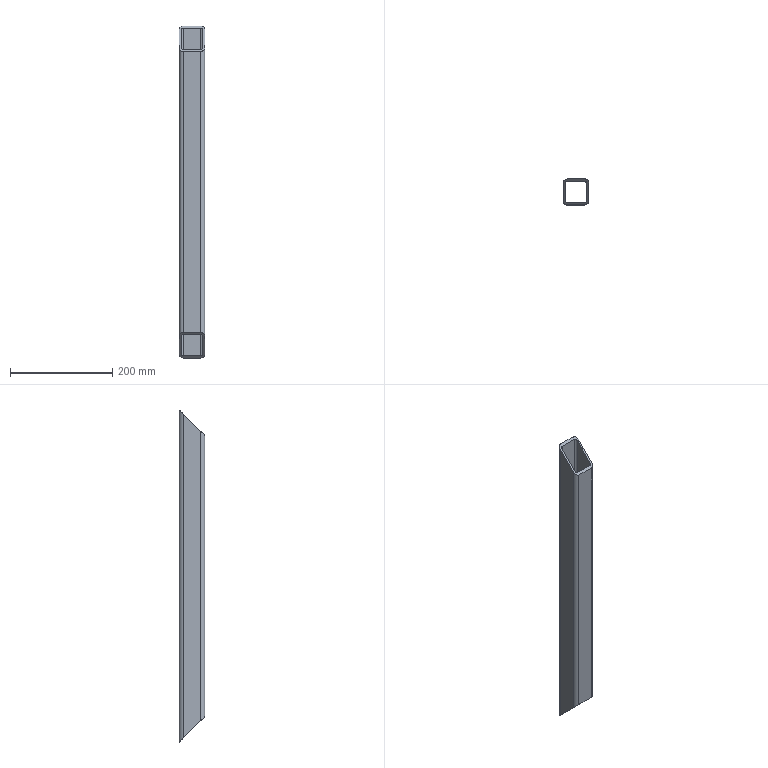Part | SolidWorks | features Extrusion 1, ICE 1, MirrorPattern 1 | 1 solid | 18 faces | box 50 x 50 x 650 mm | volume 416878 mm3 | plane 10 | cylinder 8 | commonest cylinder face diameters 8 x4 16 x4
STEP:
#1=CARTESIAN_POINT('',(17.,-25.,275.));
#2=VERTEX_POINT('',#1);
#3=CARTESIAN_POINT('',(25.,-17.,283.));
#4=VERTEX_POINT('',#3);
#5=CARTESIAN_POINT('',(17.,-25.,275.));
#6=CARTESIAN_POINT('',(21.686,-25.,275.));
#7=CARTESIAN_POINT('',(25.,-21.686,278.314));
#8=CARTESIAN_POINT('',(25.,-17.,283.));
#9=(BOUNDED_CURVE()B_SPLINE_CURVE(3,(#5,#6,#7,#8),.UNSPECIFIED.,.F.,.T.)B_SPLINE_CURVE_WITH_KNOTS((4,4),(0.,1.571),.UNSPECIFIED.)CURVE()GEOMETRIC_REPRESENTATION_ITEM()RATIONAL_B_SPLINE_CURVE((1.,0.8047,0.8047,1.))REPRESENTATION_ITEM(''));
#10=EDGE_CURVE('',#2,#4,#9,.T.);
#11=ORIENTED_EDGE('',*,*,#10,.F.);
#12=CARTESIAN_POINT('',(17.,-25.,-275.));
#13=VERTEX_POINT('',#12);
#14=CARTESIAN_POINT('',(17.,-25.,325.));
#15=DIRECTION('',(0.,0.,-1.));
#16=VECTOR('',#15,1000.);
#17=LINE('',#14,#16);
#18=EDGE_CURVE('',#2,#13,#17,.T.);
#19=ORIENTED_EDGE('',*,*,#18,.T.);
#20=CARTESIAN_POINT('',(25.,-17.,-283.));
#21=VERTEX_POINT('',#20);
#22=CARTESIAN_POINT('',(17.,-25.,-275.));
#23=CARTESIAN_POINT('',(21.686,-25.,-275.));
#24=CARTESIAN_POINT('',(25.,-21.686,-278.314));
#25=CARTESIAN_POINT('',(25.,-17.,-283.));
#26=(BOUNDED_CURVE()B_SPLINE_CURVE(3,(#22,#23,#24,#25),.UNSPECIFIED.,.F.,.T.)B_SPLINE_CURVE_WITH_KNOTS((4,4),(3.142,4.712),.UNSPECIFIED.)CURVE()GEOMETRIC_REPRESENTATION_ITEM()RATIONAL_B_SPLINE_CURVE((1.,0.8047,0.8047,1.))REPRESENTATION_ITEM(''));
#27=EDGE_CURVE('',#13,#21,#26,.T.);
#28=ORIENTED_EDGE('',*,*,#27,.T.);
#29=CARTESIAN_POINT('',(25.,-17.,325.));
#30=DIRECTION('',(0.,0.,-1.));
#31=VECTOR('',#30,1000.);
#32=LINE('',#29,#31);
#33=EDGE_CURVE('',#4,#21,#32,.T.);
#34=ORIENTED_EDGE('',*,*,#33,.F.);
#35=EDGE_LOOP('',(#11,#19,#28,#34));
#36=FACE_OUTER_BOUND('',#35,.T.);
#37=CARTESIAN_POINT('',(17.,-17.,325.));
#38=DIRECTION('',(0.,0.,-1.));
#39=DIRECTION('',(-1.,0.,0.));
#40=AXIS2_PLACEMENT_3D('',#37,#38,#39);
#41=CYLINDRICAL_SURFACE('',#40,8.);
#42=ADVANCED_FACE('',(#36),#41,.T.);
#43=CARTESIAN_POINT('',(25.,17.,317.));
#44=VERTEX_POINT('',#43);
#45=CARTESIAN_POINT('',(25.,25.,325.));
#46=DIRECTION('',(0.,0.7071,0.7071));
#47=VECTOR('',#46,1000.);
#48=LINE('',#45,#47);
#49=EDGE_CURVE('',#4,#44,#48,.T.);
#50=ORIENTED_EDGE('',*,*,#49,.F.);
#51=ORIENTED_EDGE('',*,*,#33,.T.);
#52=CARTESIAN_POINT('',(25.,17.,-317.));
#53=VERTEX_POINT('',#52);
#54=CARTESIAN_POINT('',(25.,25.,-325.));
#55=DIRECTION('',(0.,0.7071,-0.7071));
#56=VECTOR('',#55,1000.);
#57=LINE('',#54,#56);
#58=EDGE_CURVE('',#21,#53,#57,.T.);
#59=ORIENTED_EDGE('',*,*,#58,.T.);
#60=CARTESIAN_POINT('',(25.,17.,325.));
#61=DIRECTION('',(0.,0.,-1.));
#62=VECTOR('',#61,1000.);
#63=LINE('',#60,#62);
#64=EDGE_CURVE('',#44,#53,#63,.T.);
#65=ORIENTED_EDGE('',*,*,#64,.F.);
#66=EDGE_LOOP('',(#50,#51,#59,#65));
#67=FACE_OUTER_BOUND('',#66,.T.);
#68=CARTESIAN_POINT('',(25.,-17.,325.));
#69=DIRECTION('',(-1.,0.,0.));
#70=DIRECTION('',(0.,0.,1.));
#71=AXIS2_PLACEMENT_3D('',#68,#69,#70);
#72=PLANE('',#71);
#73=ADVANCED_FACE('',(#67),#72,.F.);
#74=CARTESIAN_POINT('',(17.,25.,325.));
#75=VERTEX_POINT('',#74);
#76=CARTESIAN_POINT('',(25.,17.,317.));
#77=CARTESIAN_POINT('',(25.,21.686,321.686));
#78=CARTESIAN_POINT('',(21.686,25.,325.));
#79=CARTESIAN_POINT('',(17.,25.,325.));
#80=(BOUNDED_CURVE()B_SPLINE_CURVE(3,(#76,#77,#78,#79),.UNSPECIFIED.,.F.,.T.)B_SPLINE_CURVE_WITH_KNOTS((4,4),(1.571,3.142),.UNSPECIFIED.)CURVE()GEOMETRIC_REPRESENTATION_ITEM()RATIONAL_B_SPLINE_CURVE((1.,0.8047,0.8047,1.))REPRESENTATION_ITEM(''));
#81=EDGE_CURVE('',#44,#75,#80,.T.);
#82=ORIENTED_EDGE('',*,*,#81,.F.);
#83=ORIENTED_EDGE('',*,*,#64,.T.);
#84=CARTESIAN_POINT('',(17.,25.,-325.));
#85=VERTEX_POINT('',#84);
#86=CARTESIAN_POINT('',(25.,17.,-317.));
#87=CARTESIAN_POINT('',(25.,21.686,-321.686));
#88=CARTESIAN_POINT('',(21.686,25.,-325.));
#89=CARTESIAN_POINT('',(17.,25.,-325.));
#90=(BOUNDED_CURVE()B_SPLINE_CURVE(3,(#86,#87,#88,#89),.UNSPECIFIED.,.F.,.T.)B_SPLINE_CURVE_WITH_KNOTS((4,4),(4.712,6.283),.UNSPECIFIED.)CURVE()GEOMETRIC_REPRESENTATION_ITEM()RATIONAL_B_SPLINE_CURVE((1.,0.8047,0.8047,1.))REPRESENTATION_ITEM(''));
#91=EDGE_CURVE('',#53,#85,#90,.T.);
#92=ORIENTED_EDGE('',*,*,#91,.T.);
#93=CARTESIAN_POINT('',(17.,25.,325.));
#94=DIRECTION('',(0.,0.,-1.));
#95=VECTOR('',#94,1000.);
#96=LINE('',#93,#95);
#97=EDGE_CURVE('',#75,#85,#96,.T.);
#98=ORIENTED_EDGE('',*,*,#97,.F.);
#99=EDGE_LOOP('',(#82,#83,#92,#98));
#100=FACE_OUTER_BOUND('',#99,.T.);
#101=CARTESIAN_POINT('',(17.,17.,325.));
#102=DIRECTION('',(0.,0.,-1.));
#103=DIRECTION('',(-1.,0.,0.));
#104=AXIS2_PLACEMENT_3D('',#101,#102,#103);
#105=CYLINDRICAL_SURFACE('',#104,8.);
#106=ADVANCED_FACE('',(#100),#105,.T.);
#107=CARTESIAN_POINT('',(-17.,25.,325.));
#108=VERTEX_POINT('',#107);
#109=CARTESIAN_POINT('',(-25.,17.,317.));
#110=VERTEX_POINT('',#109);
#111=CARTESIAN_POINT('',(-17.,25.,325.));
#112=CARTESIAN_POINT('',(-21.686,25.,325.));
#113=CARTESIAN_POINT('',(-25.,21.686,321.686));
#114=CARTESIAN_POINT('',(-25.,17.,317.));
#115=(BOUNDED_CURVE()B_SPLINE_CURVE(3,(#111,#112,#113,#114),.UNSPECIFIED.,.F.,.T.)B_SPLINE_CURVE_WITH_KNOTS((4,4),(3.142,4.712),.UNSPECIFIED.)CURVE()GEOMETRIC_REPRESENTATION_ITEM()RATIONAL_B_SPLINE_CURVE((1.,0.8047,0.8047,1.))REPRESENTATION_ITEM(''));
#116=EDGE_CURVE('',#108,#110,#115,.T.);
#117=ORIENTED_EDGE('',*,*,#116,.F.);
#118=CARTESIAN_POINT('',(-17.,25.,-325.));
#119=VERTEX_POINT('',#118);
#120=CARTESIAN_POINT('',(-17.,25.,325.));
#121=DIRECTION('',(0.,0.,-1.));
#122=VECTOR('',#121,1000.);
#123=LINE('',#120,#122);
#124=EDGE_CURVE('',#108,#119,#123,.T.);
#125=ORIENTED_EDGE('',*,*,#124,.T.);
#126=CARTESIAN_POINT('',(-25.,17.,-317.));
#127=VERTEX_POINT('',#126);
#128=CARTESIAN_POINT('',(-17.,25.,-325.));
#129=CARTESIAN_POINT('',(-21.686,25.,-325.));
#130=CARTESIAN_POINT('',(-25.,21.686,-321.686));
#131=CARTESIAN_POINT('',(-25.,17.,-317.));
#132=(BOUNDED_CURVE()B_SPLINE_CURVE(3,(#128,#129,#130,#131),.UNSPECIFIED.,.F.,.T.)B_SPLINE_CURVE_WITH_KNOTS((4,4),(0.,1.571),.UNSPECIFIED.)CURVE()GEOMETRIC_REPRESENTATION_ITEM()RATIONAL_B_SPLINE_CURVE((1.,0.8047,0.8047,1.))REPRESENTATION_ITEM(''));
#133=EDGE_CURVE('',#119,#127,#132,.T.);
#134=ORIENTED_EDGE('',*,*,#133,.T.);
#135=CARTESIAN_POINT('',(-25.,17.,325.));
#136=DIRECTION('',(0.,0.,-1.));
#137=VECTOR('',#136,1000.);
#138=LINE('',#135,#137);
#139=EDGE_CURVE('',#110,#127,#138,.T.);
#140=ORIENTED_EDGE('',*,*,#139,.F.);
#141=EDGE_LOOP('',(#117,#125,#134,#140));
#142=FACE_OUTER_BOUND('',#141,.T.);
#143=CARTESIAN_POINT('',(-17.,17.,325.));
#144=DIRECTION('',(0.,0.,-1.));
#145=DIRECTION('',(-1.,0.,0.));
#146=AXIS2_PLACEMENT_3D('',#143,#144,#145);
#147=CYLINDRICAL_SURFACE('',#146,8.);
#148=ADVANCED_FACE('',(#142),#147,.T.);
#149=CARTESIAN_POINT('',(-25.,-17.,283.));
#150=VERTEX_POINT('',#149);
#151=CARTESIAN_POINT('',(-25.,25.,325.));
#152=DIRECTION('',(0.,0.7071,0.7071));
#153=VECTOR('',#152,1000.);
#154=LINE('',#151,#153);
#155=EDGE_CURVE('',#150,#110,#154,.T.);
#156=ORIENTED_EDGE('',*,*,#155,.T.);
#157=ORIENTED_EDGE('',*,*,#139,.T.);
#158=CARTESIAN_POINT('',(-25.,-17.,-283.));
#159=VERTEX_POINT('',#158);
#160=CARTESIAN_POINT('',(-25.,25.,-325.));
#161=DIRECTION('',(0.,0.7071,-0.7071));
#162=VECTOR('',#161,1000.);
#163=LINE('',#160,#162);
#164=EDGE_CURVE('',#159,#127,#163,.T.);
#165=ORIENTED_EDGE('',*,*,#164,.F.);
#166=CARTESIAN_POINT('',(-25.,-17.,325.));
#167=DIRECTION('',(0.,0.,-1.));
#168=VECTOR('',#167,1000.);
#169=LINE('',#166,#168);
#170=EDGE_CURVE('',#150,#159,#169,.T.);
#171=ORIENTED_EDGE('',*,*,#170,.F.);
#172=EDGE_LOOP('',(#156,#157,#165,#171));
#173=FACE_OUTER_BOUND('',#172,.T.);
#174=CARTESIAN_POINT('',(-25.,-17.,325.));
#175=DIRECTION('',(1.,0.,0.));
#176=DIRECTION('',(0.,0.,-1.));
#177=AXIS2_PLACEMENT_3D('',#174,#175,#176);
#178=PLANE('',#177);
#179=ADVANCED_FACE('',(#173),#178,.F.);
#180=CARTESIAN_POINT('',(-17.,-25.,275.));
#181=VERTEX_POINT('',#180);
#182=CARTESIAN_POINT('',(-25.,-17.,283.));
#183=CARTESIAN_POINT('',(-25.,-21.686,278.314));
#184=CARTESIAN_POINT('',(-21.686,-25.,275.));
#185=CARTESIAN_POINT('',(-17.,-25.,275.));
#186=(BOUNDED_CURVE()B_SPLINE_CURVE(3,(#182,#183,#184,#185),.UNSPECIFIED.,.F.,.T.)B_SPLINE_CURVE_WITH_KNOTS((4,4),(4.712,6.283),.UNSPECIFIED.)CURVE()GEOMETRIC_REPRESENTATION_ITEM()RATIONAL_B_SPLINE_CURVE((1.,0.8047,0.8047,1.))REPRESENTATION_ITEM(''));
#187=EDGE_CURVE('',#150,#181,#186,.T.);
#188=ORIENTED_EDGE('',*,*,#187,.F.);
#189=ORIENTED_EDGE('',*,*,#170,.T.);
#190=CARTESIAN_POINT('',(-17.,-25.,-275.));
#191=VERTEX_POINT('',#190);
#192=CARTESIAN_POINT('',(-25.,-17.,-283.));
#193=CARTESIAN_POINT('',(-25.,-21.686,-278.314));
#194=CARTESIAN_POINT('',(-21.686,-25.,-275.));
#195=CARTESIAN_POINT('',(-17.,-25.,-275.));
#196=(BOUNDED_CURVE()B_SPLINE_CURVE(3,(#192,#193,#194,#195),.UNSPECIFIED.,.F.,.F.)B_SPLINE_CURVE_WITH_KNOTS((4,4),(1.571,3.142),.UNSPECIFIED.)CURVE()GEOMETRIC_REPRESENTATION_ITEM()RATIONAL_B_SPLINE_CURVE((1.,0.8047,0.8047,1.))REPRESENTATION_ITEM(''));
#197=EDGE_CURVE('',#159,#191,#196,.T.);
#198=ORIENTED_EDGE('',*,*,#197,.T.);
#199=CARTESIAN_POINT('',(-17.,-25.,325.));
#200=DIRECTION('',(0.,0.,-1.));
#201=VECTOR('',#200,1000.);
#202=LINE('',#199,#201);
#203=EDGE_CURVE('',#181,#191,#202,.T.);
#204=ORIENTED_EDGE('',*,*,#203,.F.);
#205=EDGE_LOOP('',(#188,#189,#198,#204));
#206=FACE_OUTER_BOUND('',#205,.T.);
#207=CARTESIAN_POINT('',(-17.,-17.,325.));
#208=DIRECTION('',(0.,0.,-1.));
#209=DIRECTION('',(-1.,0.,0.));
#210=AXIS2_PLACEMENT_3D('',#207,#208,#209);
#211=CYLINDRICAL_SURFACE('',#210,8.);
#212=ADVANCED_FACE('',(#206),#211,.T.);
#213=CARTESIAN_POINT('',(25.,-25.,275.));
#214=DIRECTION('',(-1.,0.,0.));
#215=VECTOR('',#214,1000.);
#216=LINE('',#213,#215);
#217=EDGE_CURVE('',#2,#181,#216,.T.);
#218=ORIENTED_EDGE('',*,*,#217,.T.);
#219=ORIENTED_EDGE('',*,*,#203,.T.);
#220=CARTESIAN_POINT('',(25.,-25.,-275.));
#221=DIRECTION('',(-1.,0.,0.));
#222=VECTOR('',#221,1000.);
#223=LINE('',#220,#222);
#224=EDGE_CURVE('',#13,#191,#223,.T.);
#225=ORIENTED_EDGE('',*,*,#224,.F.);
#226=ORIENTED_EDGE('',*,*,#18,.F.);
#227=EDGE_LOOP('',(#218,#219,#225,#226));
#228=FACE_OUTER_BOUND('',#227,.T.);
#229=CARTESIAN_POINT('',(-17.,-25.,325.));
#230=DIRECTION('',(0.,1.,0.));
#231=DIRECTION('',(0.,0.,1.));
#232=AXIS2_PLACEMENT_3D('',#229,#230,#231);
#233=PLANE('',#232);
#234=ADVANCED_FACE('',(#228),#233,.F.);
#235=CARTESIAN_POINT('',(-17.,21.,321.));
#236=VERTEX_POINT('',#235);
#237=CARTESIAN_POINT('',(-17.,21.,-321.));
#238=VERTEX_POINT('',#237);
#239=CARTESIAN_POINT('',(-17.,21.,325.));
#240=DIRECTION('',(0.,0.,-1.));
#241=VECTOR('',#240,1000.);
#242=LINE('',#239,#241);
#243=EDGE_CURVE('',#236,#238,#242,.T.);
#244=ORIENTED_EDGE('',*,*,#243,.F.);
#245=CARTESIAN_POINT('',(-21.,17.,317.));
#246=VERTEX_POINT('',#245);
#247=CARTESIAN_POINT('',(-17.,21.,321.));
#248=CARTESIAN_POINT('',(-19.343,21.,321.));
#249=CARTESIAN_POINT('',(-21.,19.343,319.343));
#250=CARTESIAN_POINT('',(-21.,17.,317.));
#251=(BOUNDED_CURVE()B_SPLINE_CURVE(3,(#247,#248,#249,#250),.UNSPECIFIED.,.F.,.T.)B_SPLINE_CURVE_WITH_KNOTS((4,4),(3.142,4.712),.UNSPECIFIED.)CURVE()GEOMETRIC_REPRESENTATION_ITEM()RATIONAL_B_SPLINE_CURVE((1.,0.8047,0.8047,1.))REPRESENTATION_ITEM(''));
#252=EDGE_CURVE('',#236,#246,#251,.T.);
#253=ORIENTED_EDGE('',*,*,#252,.T.);
#254=CARTESIAN_POINT('',(-21.,17.,-317.));
#255=VERTEX_POINT('',#254);
#256=CARTESIAN_POINT('',(-21.,17.,325.));
#257=DIRECTION('',(0.,0.,-1.));
#258=VECTOR('',#257,1000.);
#259=LINE('',#256,#258);
#260=EDGE_CURVE('',#246,#255,#259,.T.);
#261=ORIENTED_EDGE('',*,*,#260,.T.);
#262=CARTESIAN_POINT('',(-17.,21.,-321.));
#263=CARTESIAN_POINT('',(-19.343,21.,-321.));
#264=CARTESIAN_POINT('',(-21.,19.343,-319.343));
#265=CARTESIAN_POINT('',(-21.,17.,-317.));
#266=(BOUNDED_CURVE()B_SPLINE_CURVE(3,(#262,#263,#264,#265),.UNSPECIFIED.,.F.,.T.)B_SPLINE_CURVE_WITH_KNOTS((4,4),(0.,1.571),.UNSPECIFIED.)CURVE()GEOMETRIC_REPRESENTATION_ITEM()RATIONAL_B_SPLINE_CURVE((1.,0.8047,0.8047,1.))REPRESENTATION_ITEM(''));
#267=EDGE_CURVE('',#238,#255,#266,.T.);
#268=ORIENTED_EDGE('',*,*,#267,.F.);
#269=EDGE_LOOP('',(#244,#253,#261,#268));
#270=FACE_OUTER_BOUND('',#269,.T.);
#271=CARTESIAN_POINT('',(-17.,17.,325.));
#272=DIRECTION('',(0.,0.,-1.));
#273=DIRECTION('',(-1.,0.,0.));
#274=AXIS2_PLACEMENT_3D('',#271,#272,#273);
#275=CYLINDRICAL_SURFACE('',#274,4.);
#276=ADVANCED_FACE('',(#270),#275,.F.);
#277=ORIENTED_EDGE('',*,*,#260,.F.);
#278=CARTESIAN_POINT('',(-21.,-17.,283.));
#279=VERTEX_POINT('',#278);
#280=CARTESIAN_POINT('',(-21.,4.,304.));
#281=DIRECTION('',(0.,-0.7071,-0.7071));
#282=VECTOR('',#281,1000.);
#283=LINE('',#280,#282);
#284=EDGE_CURVE('',#246,#279,#283,.T.);
#285=ORIENTED_EDGE('',*,*,#284,.T.);
#286=CARTESIAN_POINT('',(-21.,-17.,-283.));
#287=VERTEX_POINT('',#286);
#288=CARTESIAN_POINT('',(-21.,-17.,325.));
#289=DIRECTION('',(0.,0.,-1.));
#290=VECTOR('',#289,1000.);
#291=LINE('',#288,#290);
#292=EDGE_CURVE('',#279,#287,#291,.T.);
#293=ORIENTED_EDGE('',*,*,#292,.T.);
#294=CARTESIAN_POINT('',(-21.,-321.,21.));
#295=DIRECTION('',(0.,-0.7071,0.7071));
#296=VECTOR('',#295,1000.);
#297=LINE('',#294,#296);
#298=EDGE_CURVE('',#255,#287,#297,.T.);
#299=ORIENTED_EDGE('',*,*,#298,.F.);
#300=EDGE_LOOP('',(#277,#285,#293,#299));
#301=FACE_OUTER_BOUND('',#300,.T.);
#302=CARTESIAN_POINT('',(-21.,-17.,325.));
#303=DIRECTION('',(1.,0.,0.));
#304=DIRECTION('',(0.,0.,-1.));
#305=AXIS2_PLACEMENT_3D('',#302,#303,#304);
#306=PLANE('',#305);
#307=ADVANCED_FACE('',(#301),#306,.T.);
#308=ORIENTED_EDGE('',*,*,#292,.F.);
#309=CARTESIAN_POINT('',(-17.,-21.,279.));
#310=VERTEX_POINT('',#309);
#311=CARTESIAN_POINT('',(-21.,-17.,283.));
#312=CARTESIAN_POINT('',(-21.,-19.343,280.657));
#313=CARTESIAN_POINT('',(-19.343,-21.,279.));
#314=CARTESIAN_POINT('',(-17.,-21.,279.));
#315=(BOUNDED_CURVE()B_SPLINE_CURVE(3,(#311,#312,#313,#314),.UNSPECIFIED.,.F.,.T.)B_SPLINE_CURVE_WITH_KNOTS((4,4),(4.712,6.283),.UNSPECIFIED.)CURVE()GEOMETRIC_REPRESENTATION_ITEM()RATIONAL_B_SPLINE_CURVE((1.,0.8047,0.8047,1.))REPRESENTATION_ITEM(''));
#316=EDGE_CURVE('',#279,#310,#315,.T.);
#317=ORIENTED_EDGE('',*,*,#316,.T.);
#318=CARTESIAN_POINT('',(-17.,-21.,-279.));
#319=VERTEX_POINT('',#318);
#320=CARTESIAN_POINT('',(-17.,-21.,325.));
#321=DIRECTION('',(0.,0.,-1.));
#322=VECTOR('',#321,1000.);
#323=LINE('',#320,#322);
#324=EDGE_CURVE('',#310,#319,#323,.T.);
#325=ORIENTED_EDGE('',*,*,#324,.T.);
#326=CARTESIAN_POINT('',(-21.,-17.,-283.));
#327=CARTESIAN_POINT('',(-21.,-19.343,-280.657));
#328=CARTESIAN_POINT('',(-19.343,-21.,-279.));
#329=CARTESIAN_POINT('',(-17.,-21.,-279.));
#330=(BOUNDED_CURVE()B_SPLINE_CURVE(3,(#326,#327,#328,#329),.UNSPECIFIED.,.F.,.T.)B_SPLINE_CURVE_WITH_KNOTS((4,4),(1.571,3.142),.UNSPECIFIED.)CURVE()GEOMETRIC_REPRESENTATION_ITEM()RATIONAL_B_SPLINE_CURVE((1.,0.8047,0.8047,1.))REPRESENTATION_ITEM(''));
#331=EDGE_CURVE('',#287,#319,#330,.T.);
#332=ORIENTED_EDGE('',*,*,#331,.F.);
#333=EDGE_LOOP('',(#308,#317,#325,#332));
#334=FACE_OUTER_BOUND('',#333,.T.);
#335=CARTESIAN_POINT('',(-17.,-17.,325.));
#336=DIRECTION('',(0.,0.,-1.));
#337=DIRECTION('',(-1.,0.,0.));
#338=AXIS2_PLACEMENT_3D('',#335,#336,#337);
#339=CYLINDRICAL_SURFACE('',#338,4.);
#340=ADVANCED_FACE('',(#334),#339,.F.);
#341=ORIENTED_EDGE('',*,*,#324,.F.);
#342=CARTESIAN_POINT('',(17.,-21.,279.));
#343=VERTEX_POINT('',#342);
#344=CARTESIAN_POINT('',(-17.,-21.,279.));
#345=DIRECTION('',(1.,0.,0.));
#346=VECTOR('',#345,1000.);
#347=LINE('',#344,#346);
#348=EDGE_CURVE('',#310,#343,#347,.T.);
#349=ORIENTED_EDGE('',*,*,#348,.T.);
#350=CARTESIAN_POINT('',(17.,-21.,-279.));
#351=VERTEX_POINT('',#350);
#352=CARTESIAN_POINT('',(17.,-21.,325.));
#353=DIRECTION('',(0.,0.,-1.));
#354=VECTOR('',#353,1000.);
#355=LINE('',#352,#354);
#356=EDGE_CURVE('',#343,#351,#355,.T.);
#357=ORIENTED_EDGE('',*,*,#356,.T.);
#358=CARTESIAN_POINT('',(-17.,-21.,-279.));
#359=DIRECTION('',(1.,0.,0.));
#360=VECTOR('',#359,1000.);
#361=LINE('',#358,#360);
#362=EDGE_CURVE('',#319,#351,#361,.T.);
#363=ORIENTED_EDGE('',*,*,#362,.F.);
#364=EDGE_LOOP('',(#341,#349,#357,#363));
#365=FACE_OUTER_BOUND('',#364,.T.);
#366=CARTESIAN_POINT('',(-17.,-21.,325.));
#367=DIRECTION('',(0.,1.,0.));
#368=DIRECTION('',(0.,0.,1.));
#369=AXIS2_PLACEMENT_3D('',#366,#367,#368);
#370=PLANE('',#369);
#371=ADVANCED_FACE('',(#365),#370,.T.);
#372=ORIENTED_EDGE('',*,*,#356,.F.);
#373=CARTESIAN_POINT('',(21.,-17.,283.));
#374=VERTEX_POINT('',#373);
#375=CARTESIAN_POINT('',(17.,-21.,279.));
#376=CARTESIAN_POINT('',(19.343,-21.,279.));
#377=CARTESIAN_POINT('',(21.,-19.343,280.657));
#378=CARTESIAN_POINT('',(21.,-17.,283.));
#379=(BOUNDED_CURVE()B_SPLINE_CURVE(3,(#375,#376,#377,#378),.UNSPECIFIED.,.F.,.F.)B_SPLINE_CURVE_WITH_KNOTS((4,4),(0.,1.571),.UNSPECIFIED.)CURVE()GEOMETRIC_REPRESENTATION_ITEM()RATIONAL_B_SPLINE_CURVE((1.,0.8047,0.8047,1.))REPRESENTATION_ITEM(''));
#380=EDGE_CURVE('',#343,#374,#379,.T.);
#381=ORIENTED_EDGE('',*,*,#380,.T.);
#382=CARTESIAN_POINT('',(21.,-17.,-283.));
#383=VERTEX_POINT('',#382);
#384=CARTESIAN_POINT('',(21.,-17.,325.));
#385=DIRECTION('',(0.,0.,-1.));
#386=VECTOR('',#385,1000.);
#387=LINE('',#384,#386);
#388=EDGE_CURVE('',#374,#383,#387,.T.);
#389=ORIENTED_EDGE('',*,*,#388,.T.);
#390=CARTESIAN_POINT('',(17.,-21.,-279.));
#391=CARTESIAN_POINT('',(19.343,-21.,-279.));
#392=CARTESIAN_POINT('',(21.,-19.343,-280.657));
#393=CARTESIAN_POINT('',(21.,-17.,-283.));
#394=(BOUNDED_CURVE()B_SPLINE_CURVE(3,(#390,#391,#392,#393),.UNSPECIFIED.,.F.,.F.)B_SPLINE_CURVE_WITH_KNOTS((4,4),(3.142,4.712),.UNSPECIFIED.)CURVE()GEOMETRIC_REPRESENTATION_ITEM()RATIONAL_B_SPLINE_CURVE((1.,0.8047,0.8047,1.))REPRESENTATION_ITEM(''));
#395=EDGE_CURVE('',#351,#383,#394,.T.);
#396=ORIENTED_EDGE('',*,*,#395,.F.);
#397=EDGE_LOOP('',(#372,#381,#389,#396));
#398=FACE_OUTER_BOUND('',#397,.T.);
#399=CARTESIAN_POINT('',(17.,-17.,325.));
#400=DIRECTION('',(0.,0.,-1.));
#401=DIRECTION('',(-1.,0.,0.));
#402=AXIS2_PLACEMENT_3D('',#399,#400,#401);
#403=CYLINDRICAL_SURFACE('',#402,4.);
#404=ADVANCED_FACE('',(#398),#403,.F.);
#405=ORIENTED_EDGE('',*,*,#388,.F.);
#406=CARTESIAN_POINT('',(21.,17.,317.));
#407=VERTEX_POINT('',#406);
#408=CARTESIAN_POINT('',(21.,4.,304.));
#409=DIRECTION('',(0.,0.7071,0.7071));
#410=VECTOR('',#409,1000.);
#411=LINE('',#408,#410);
#412=EDGE_CURVE('',#374,#407,#411,.T.);
#413=ORIENTED_EDGE('',*,*,#412,.T.);
#414=CARTESIAN_POINT('',(21.,17.,-317.));
#415=VERTEX_POINT('',#414);
#416=CARTESIAN_POINT('',(21.,17.,325.));
#417=DIRECTION('',(0.,0.,-1.));
#418=VECTOR('',#417,1000.);
#419=LINE('',#416,#418);
#420=EDGE_CURVE('',#407,#415,#419,.T.);
#421=ORIENTED_EDGE('',*,*,#420,.T.);
#422=CARTESIAN_POINT('',(21.,-321.,21.));
#423=DIRECTION('',(0.,0.7071,-0.7071));
#424=VECTOR('',#423,1000.);
#425=LINE('',#422,#424);
#426=EDGE_CURVE('',#383,#415,#425,.T.);
#427=ORIENTED_EDGE('',*,*,#426,.F.);
#428=EDGE_LOOP('',(#405,#413,#421,#427));
#429=FACE_OUTER_BOUND('',#428,.T.);
#430=CARTESIAN_POINT('',(21.,-17.,325.));
#431=DIRECTION('',(-1.,0.,0.));
#432=DIRECTION('',(0.,0.,1.));
#433=AXIS2_PLACEMENT_3D('',#430,#431,#432);
#434=PLANE('',#433);
#435=ADVANCED_FACE('',(#429),#434,.T.);
#436=ORIENTED_EDGE('',*,*,#420,.F.);
#437=CARTESIAN_POINT('',(17.,21.,321.));
#438=VERTEX_POINT('',#437);
#439=CARTESIAN_POINT('',(21.,17.,317.));
#440=CARTESIAN_POINT('',(21.,19.343,319.343));
#441=CARTESIAN_POINT('',(19.343,21.,321.));
#442=CARTESIAN_POINT('',(17.,21.,321.));
#443=(BOUNDED_CURVE()B_SPLINE_CURVE(3,(#439,#440,#441,#442),.UNSPECIFIED.,.F.,.T.)B_SPLINE_CURVE_WITH_KNOTS((4,4),(1.571,3.142),.UNSPECIFIED.)CURVE()GEOMETRIC_REPRESENTATION_ITEM()RATIONAL_B_SPLINE_CURVE((1.,0.8047,0.8047,1.))REPRESENTATION_ITEM(''));
#444=EDGE_CURVE('',#407,#438,#443,.T.);
#445=ORIENTED_EDGE('',*,*,#444,.T.);
#446=CARTESIAN_POINT('',(17.,21.,-321.));
#447=VERTEX_POINT('',#446);
#448=CARTESIAN_POINT('',(17.,21.,325.));
#449=DIRECTION('',(0.,0.,-1.));
#450=VECTOR('',#449,1000.);
#451=LINE('',#448,#450);
#452=EDGE_CURVE('',#438,#447,#451,.T.);
#453=ORIENTED_EDGE('',*,*,#452,.T.);
#454=CARTESIAN_POINT('',(21.,17.,-317.));
#455=CARTESIAN_POINT('',(21.,19.343,-319.343));
#456=CARTESIAN_POINT('',(19.343,21.,-321.));
#457=CARTESIAN_POINT('',(17.,21.,-321.));
#458=(BOUNDED_CURVE()B_SPLINE_CURVE(3,(#454,#455,#456,#457),.UNSPECIFIED.,.F.,.F.)B_SPLINE_CURVE_WITH_KNOTS((4,4),(4.712,6.283),.UNSPECIFIED.)CURVE()GEOMETRIC_REPRESENTATION_ITEM()RATIONAL_B_SPLINE_CURVE((1.,0.8047,0.8047,1.))REPRESENTATION_ITEM(''));
#459=EDGE_CURVE('',#415,#447,#458,.T.);
#460=ORIENTED_EDGE('',*,*,#459,.F.);
#461=EDGE_LOOP('',(#436,#445,#453,#460));
#462=FACE_OUTER_BOUND('',#461,.T.);
#463=CARTESIAN_POINT('',(17.,17.,325.));
#464=DIRECTION('',(0.,0.,-1.));
#465=DIRECTION('',(-1.,0.,0.));
#466=AXIS2_PLACEMENT_3D('',#463,#464,#465);
#467=CYLINDRICAL_SURFACE('',#466,4.);
#468=ADVANCED_FACE('',(#462),#467,.F.);
#469=ORIENTED_EDGE('',*,*,#452,.F.);
#470=CARTESIAN_POINT('',(-17.,21.,321.));
#471=DIRECTION('',(-1.,0.,0.));
#472=VECTOR('',#471,1000.);
#473=LINE('',#470,#472);
#474=EDGE_CURVE('',#438,#236,#473,.T.);
#475=ORIENTED_EDGE('',*,*,#474,.T.);
#476=ORIENTED_EDGE('',*,*,#243,.T.);
#477=CARTESIAN_POINT('',(-17.,21.,-321.));
#478=DIRECTION('',(-1.,0.,0.));
#479=VECTOR('',#478,1000.);
#480=LINE('',#477,#479);
#481=EDGE_CURVE('',#447,#238,#480,.T.);
#482=ORIENTED_EDGE('',*,*,#481,.F.);
#483=EDGE_LOOP('',(#469,#475,#476,#482));
#484=FACE_OUTER_BOUND('',#483,.T.);
#485=CARTESIAN_POINT('',(-17.,21.,325.));
#486=DIRECTION('',(0.,-1.,0.));
#487=DIRECTION('',(0.,0.,-1.));
#488=AXIS2_PLACEMENT_3D('',#485,#486,#487);
#489=PLANE('',#488);
#490=ADVANCED_FACE('',(#484),#489,.T.);
#491=CARTESIAN_POINT('',(-17.,25.,-325.));
#492=DIRECTION('',(-1.,0.,0.));
#493=VECTOR('',#492,1000.);
#494=LINE('',#491,#493);
#495=EDGE_CURVE('',#85,#119,#494,.T.);
#496=ORIENTED_EDGE('',*,*,#495,.T.);
#497=ORIENTED_EDGE('',*,*,#124,.F.);
#498=CARTESIAN_POINT('',(-17.,25.,325.));
#499=DIRECTION('',(-1.,0.,0.));
#500=VECTOR('',#499,1000.);
#501=LINE('',#498,#500);
#502=EDGE_CURVE('',#75,#108,#501,.T.);
#503=ORIENTED_EDGE('',*,*,#502,.F.);
#504=ORIENTED_EDGE('',*,*,#97,.T.);
#505=EDGE_LOOP('',(#496,#497,#503,#504));
#506=FACE_OUTER_BOUND('',#505,.T.);
#507=CARTESIAN_POINT('',(-17.,25.,325.));
#508=DIRECTION('',(0.,-1.,0.));
#509=DIRECTION('',(0.,0.,-1.));
#510=AXIS2_PLACEMENT_3D('',#507,#508,#509);
#511=PLANE('',#510);
#512=ADVANCED_FACE('',(#506),#511,.F.);
#513=ORIENTED_EDGE('',*,*,#267,.T.);
#514=ORIENTED_EDGE('',*,*,#298,.T.);
#515=ORIENTED_EDGE('',*,*,#331,.T.);
#516=ORIENTED_EDGE('',*,*,#362,.T.);
#517=ORIENTED_EDGE('',*,*,#395,.T.);
#518=ORIENTED_EDGE('',*,*,#426,.T.);
#519=ORIENTED_EDGE('',*,*,#459,.T.);
#520=ORIENTED_EDGE('',*,*,#481,.T.);
#521=EDGE_LOOP('',(#513,#514,#515,#516,#517,#518,#519,#520));
#522=FACE_BOUND('',#521,.T.);
#523=ORIENTED_EDGE('',*,*,#224,.T.);
#524=ORIENTED_EDGE('',*,*,#197,.F.);
#525=ORIENTED_EDGE('',*,*,#164,.T.);
#526=ORIENTED_EDGE('',*,*,#133,.F.);
#527=ORIENTED_EDGE('',*,*,#495,.F.);
#528=ORIENTED_EDGE('',*,*,#91,.F.);
#529=ORIENTED_EDGE('',*,*,#58,.F.);
#530=ORIENTED_EDGE('',*,*,#27,.F.);
#531=EDGE_LOOP('',(#523,#524,#525,#526,#527,#528,#529,#530));
#532=FACE_OUTER_BOUND('',#531,.T.);
#533=CARTESIAN_POINT('',(25.,25.,-325.));
#534=DIRECTION('',(0.,0.7071,0.7071));
#535=DIRECTION('',(0.,-0.7071,0.7071));
#536=AXIS2_PLACEMENT_3D('',#533,#534,#535);
#537=PLANE('',#536);
#538=ADVANCED_FACE('',(#522,#532),#537,.F.);
#539=ORIENTED_EDGE('',*,*,#474,.F.);
#540=ORIENTED_EDGE('',*,*,#444,.F.);
#541=ORIENTED_EDGE('',*,*,#412,.F.);
#542=ORIENTED_EDGE('',*,*,#380,.F.);
#543=ORIENTED_EDGE('',*,*,#348,.F.);
#544=ORIENTED_EDGE('',*,*,#316,.F.);
#545=ORIENTED_EDGE('',*,*,#284,.F.);
#546=ORIENTED_EDGE('',*,*,#252,.F.);
#547=EDGE_LOOP('',(#539,#540,#541,#542,#543,#544,#545,#546));
#548=FACE_BOUND('',#547,.T.);
#549=ORIENTED_EDGE('',*,*,#10,.T.);
#550=ORIENTED_EDGE('',*,*,#49,.T.);
#551=ORIENTED_EDGE('',*,*,#81,.T.);
#552=ORIENTED_EDGE('',*,*,#502,.T.);
#553=ORIENTED_EDGE('',*,*,#116,.T.);
#554=ORIENTED_EDGE('',*,*,#155,.F.);
#555=ORIENTED_EDGE('',*,*,#187,.T.);
#556=ORIENTED_EDGE('',*,*,#217,.F.);
#557=EDGE_LOOP('',(#549,#550,#551,#552,#553,#554,#555,#556));
#558=FACE_OUTER_BOUND('',#557,.T.);
#559=CARTESIAN_POINT('',(25.,25.,325.));
#560=DIRECTION('',(0.,-0.7071,0.7071));
#561=DIRECTION('',(0.,-0.7071,-0.7071));
#562=AXIS2_PLACEMENT_3D('',#559,#560,#561);
#563=PLANE('',#562);
#564=ADVANCED_FACE('',(#548,#558),#563,.T.);
#565=CLOSED_SHELL('',(#42,#73,#106,#148,#179,#212,#234,#276,#307,#340,#371,#404,#435,#468,#490,#512,#538,#564));
#566=MANIFOLD_SOLID_BREP('',#565);
#567=CARTESIAN_POINT('',(0.,0.,0.));
#568=DIRECTION('',(0.,0.,1.));
#569=DIRECTION('',(1.,0.,0.));
#570=AXIS2_PLACEMENT_3D('',#567,#568,#569);
#571=(LENGTH_UNIT()NAMED_UNIT(*)SI_UNIT(.MILLI.,.METRE.));
#572=UNCERTAINTY_MEASURE_WITH_UNIT(LENGTH_MEASURE(0.00001),#571,'','');
#573=(NAMED_UNIT(*)PLANE_ANGLE_UNIT()SI_UNIT($,.RADIAN.));
#574=(NAMED_UNIT(*)SI_UNIT($,.STERADIAN.)SOLID_ANGLE_UNIT());
#575=(GEOMETRIC_REPRESENTATION_CONTEXT(3)GLOBAL_UNCERTAINTY_ASSIGNED_CONTEXT((#572))GLOBAL_UNIT_ASSIGNED_CONTEXT((#571,#573,#574))REPRESENTATION_CONTEXT('',''));
#576=ADVANCED_BREP_SHAPE_REPRESENTATION('',(#566,#570),#575);